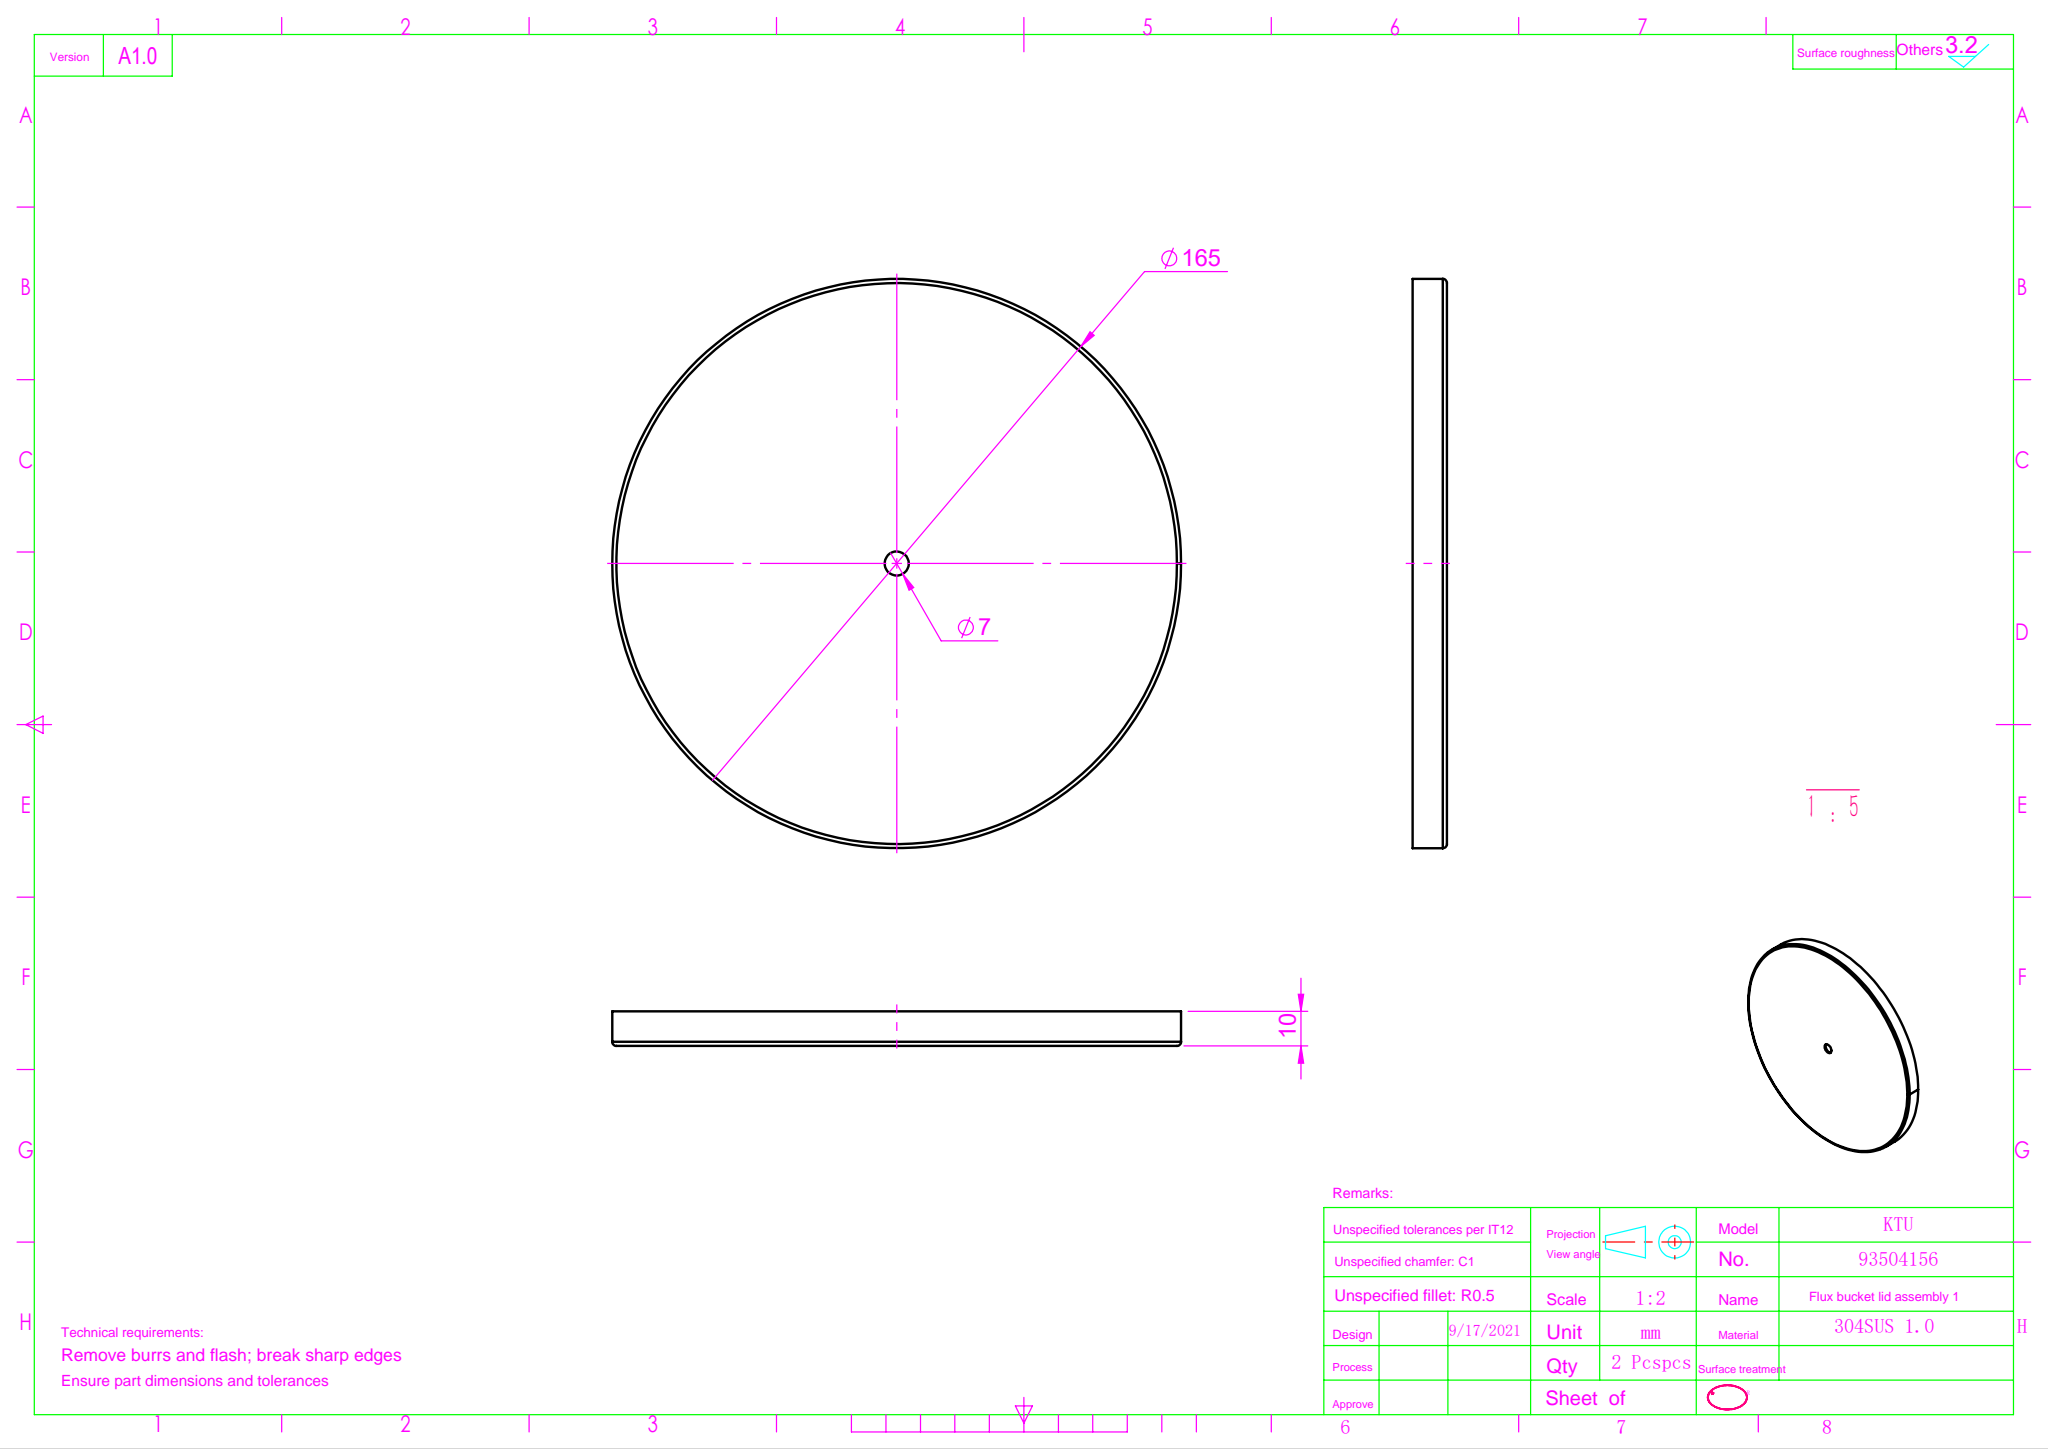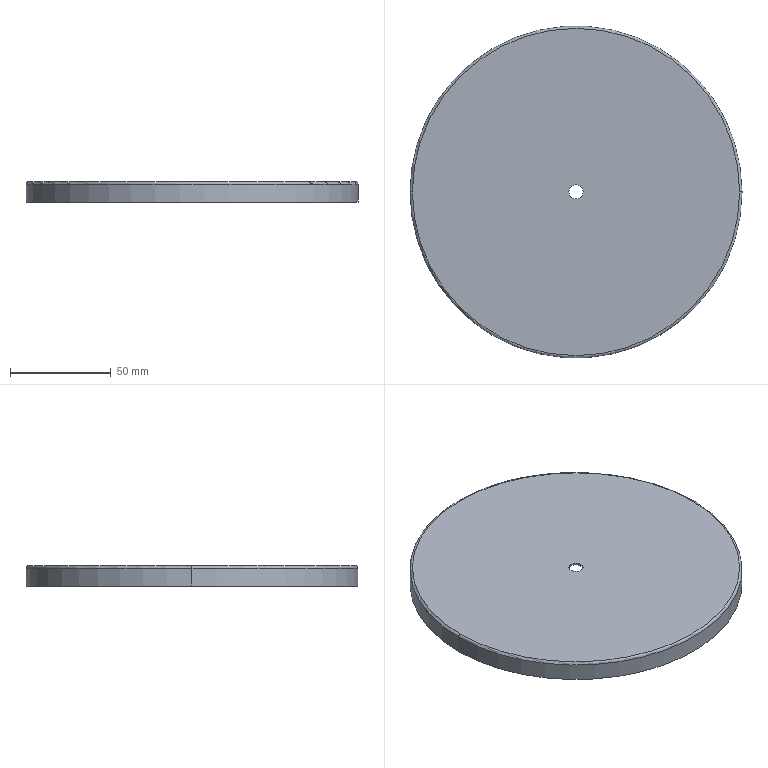Part | SolidWorks | features 3DProfileFeature 1, EdgeFlange 1, FlatPattern 1, ICE 1, SMBaseFlange 1, SheetMetal 1 | 1 solid | 13 faces | box 165 x 165 x 10 mm | volume 25826 mm3 | cylinder 6 | torus 4 | plane 3 | commonest cylinder face diameters 7 x2 163 x2 165 x2
STEP:
#1=CARTESIAN_POINT('',(-3.5,0.,-1.));
#2=VERTEX_POINT('',#1);
#3=CARTESIAN_POINT('',(3.5,0.,-1.));
#4=VERTEX_POINT('',#3);
#5=CARTESIAN_POINT('',(0.,0.,-1.));
#6=DIRECTION('',(0.,0.,1.));
#7=DIRECTION('',(1.,0.,0.));
#8=AXIS2_PLACEMENT_3D('',#5,#6,#7);
#9=CIRCLE('',#8,3.5);
#10=EDGE_CURVE('',#2,#4,#9,.T.);
#11=ORIENTED_EDGE('',*,*,#10,.F.);
#12=CARTESIAN_POINT('',(-3.5,0.,0.));
#13=VERTEX_POINT('',#12);
#14=CARTESIAN_POINT('',(-3.5,0.,-10.));
#15=DIRECTION('',(0.,0.,1.));
#16=VECTOR('',#15,1000.);
#17=LINE('',#14,#16);
#18=EDGE_CURVE('',#2,#13,#17,.T.);
#19=ORIENTED_EDGE('',*,*,#18,.T.);
#20=CARTESIAN_POINT('',(3.5,0.,0.));
#21=VERTEX_POINT('',#20);
#22=CARTESIAN_POINT('',(0.,0.,0.));
#23=DIRECTION('',(0.,0.,1.));
#24=DIRECTION('',(1.,0.,0.));
#25=AXIS2_PLACEMENT_3D('',#22,#23,#24);
#26=CIRCLE('',#25,3.5);
#27=EDGE_CURVE('',#13,#21,#26,.T.);
#28=ORIENTED_EDGE('',*,*,#27,.T.);
#29=CARTESIAN_POINT('',(3.5,0.,-10.));
#30=DIRECTION('',(0.,0.,1.));
#31=VECTOR('',#30,1000.);
#32=LINE('',#29,#31);
#33=EDGE_CURVE('',#4,#21,#32,.T.);
#34=ORIENTED_EDGE('',*,*,#33,.F.);
#35=EDGE_LOOP('',(#11,#19,#28,#34));
#36=FACE_OUTER_BOUND('',#35,.T.);
#37=CARTESIAN_POINT('',(0.,0.,-10.));
#38=DIRECTION('',(0.,0.,1.));
#39=DIRECTION('',(1.,0.,0.));
#40=AXIS2_PLACEMENT_3D('',#37,#38,#39);
#41=CYLINDRICAL_SURFACE('',#40,3.5);
#42=ADVANCED_FACE('',(#36),#41,.F.);
#43=CARTESIAN_POINT('',(-81.5,0.,-1.2));
#44=VERTEX_POINT('',#43);
#45=CARTESIAN_POINT('',(81.5,0.,-1.2));
#46=VERTEX_POINT('',#45);
#47=CARTESIAN_POINT('',(0.,0.,-1.2));
#48=DIRECTION('',(0.,0.,1.));
#49=DIRECTION('',(1.,0.,0.));
#50=AXIS2_PLACEMENT_3D('',#47,#48,#49);
#51=CIRCLE('',#50,81.5);
#52=EDGE_CURVE('',#44,#46,#51,.T.);
#53=ORIENTED_EDGE('',*,*,#52,.F.);
#54=CARTESIAN_POINT('',(-81.3,0.,-1.));
#55=VERTEX_POINT('',#54);
#56=CARTESIAN_POINT('',(-81.3,0.,-1.2));
#57=DIRECTION('',(0.,1.,0.));
#58=DIRECTION('',(-1.,0.,0.));
#59=AXIS2_PLACEMENT_3D('',#56,#57,#58);
#60=CIRCLE('',#59,0.2);
#61=EDGE_CURVE('',#44,#55,#60,.T.);
#62=ORIENTED_EDGE('',*,*,#61,.T.);
#63=CARTESIAN_POINT('',(81.3,0.,-1.));
#64=VERTEX_POINT('',#63);
#65=CARTESIAN_POINT('',(0.,0.,-1.));
#66=DIRECTION('',(0.,0.,1.));
#67=DIRECTION('',(1.,0.,0.));
#68=AXIS2_PLACEMENT_3D('',#65,#66,#67);
#69=CIRCLE('',#68,81.3);
#70=EDGE_CURVE('',#55,#64,#69,.T.);
#71=ORIENTED_EDGE('',*,*,#70,.T.);
#72=CARTESIAN_POINT('',(81.3,0.,-1.2));
#73=DIRECTION('',(0.,-1.,0.));
#74=DIRECTION('',(0.,0.,-1.));
#75=AXIS2_PLACEMENT_3D('',#72,#73,#74);
#76=CIRCLE('',#75,0.2);
#77=EDGE_CURVE('',#46,#64,#76,.T.);
#78=ORIENTED_EDGE('',*,*,#77,.F.);
#79=EDGE_LOOP('',(#53,#62,#71,#78));
#80=FACE_OUTER_BOUND('',#79,.T.);
#81=CARTESIAN_POINT('',(0.,0.,-1.2));
#82=DIRECTION('',(0.,0.,1.));
#83=DIRECTION('',(1.,0.,0.));
#84=AXIS2_PLACEMENT_3D('',#81,#82,#83);
#85=TOROIDAL_SURFACE('',#84,81.3,0.2);
#86=ADVANCED_FACE('',(#80),#85,.F.);
#87=CARTESIAN_POINT('',(-81.5,0.,-10.));
#88=VERTEX_POINT('',#87);
#89=CARTESIAN_POINT('',(81.5,0.,-10.));
#90=VERTEX_POINT('',#89);
#91=CARTESIAN_POINT('',(0.,0.,-10.));
#92=DIRECTION('',(0.,0.,1.));
#93=DIRECTION('',(1.,0.,0.));
#94=AXIS2_PLACEMENT_3D('',#91,#92,#93);
#95=CIRCLE('',#94,81.5);
#96=EDGE_CURVE('',#88,#90,#95,.T.);
#97=ORIENTED_EDGE('',*,*,#96,.F.);
#98=CARTESIAN_POINT('',(-81.5,0.,-1.));
#99=DIRECTION('',(0.,0.,1.));
#100=VECTOR('',#99,1000.);
#101=LINE('',#98,#100);
#102=EDGE_CURVE('',#88,#44,#101,.T.);
#103=ORIENTED_EDGE('',*,*,#102,.T.);
#104=ORIENTED_EDGE('',*,*,#52,.T.);
#105=CARTESIAN_POINT('',(81.5,0.,-1.));
#106=DIRECTION('',(0.,0.,1.));
#107=VECTOR('',#106,1000.);
#108=LINE('',#105,#107);
#109=EDGE_CURVE('',#90,#46,#108,.T.);
#110=ORIENTED_EDGE('',*,*,#109,.F.);
#111=EDGE_LOOP('',(#97,#103,#104,#110));
#112=FACE_OUTER_BOUND('',#111,.T.);
#113=CARTESIAN_POINT('',(0.,0.,-1.));
#114=DIRECTION('',(0.,0.,1.));
#115=DIRECTION('',(1.,0.,0.));
#116=AXIS2_PLACEMENT_3D('',#113,#114,#115);
#117=CYLINDRICAL_SURFACE('',#116,81.5);
#118=ADVANCED_FACE('',(#112),#117,.F.);
#119=CARTESIAN_POINT('',(82.5,0.,-1.2));
#120=VERTEX_POINT('',#119);
#121=CARTESIAN_POINT('',(-82.5,0.,-1.2));
#122=VERTEX_POINT('',#121);
#123=CARTESIAN_POINT('',(0.,0.,-1.2));
#124=DIRECTION('',(0.,0.,1.));
#125=DIRECTION('',(1.,0.,0.));
#126=AXIS2_PLACEMENT_3D('',#123,#124,#125);
#127=CIRCLE('',#126,82.5);
#128=EDGE_CURVE('',#120,#122,#127,.T.);
#129=ORIENTED_EDGE('',*,*,#128,.T.);
#130=CARTESIAN_POINT('',(-81.3,0.,0.));
#131=VERTEX_POINT('',#130);
#132=CARTESIAN_POINT('',(-81.3,0.,-1.2));
#133=DIRECTION('',(0.,1.,0.));
#134=DIRECTION('',(-1.,0.,0.));
#135=AXIS2_PLACEMENT_3D('',#132,#133,#134);
#136=CIRCLE('',#135,1.2);
#137=EDGE_CURVE('',#122,#131,#136,.T.);
#138=ORIENTED_EDGE('',*,*,#137,.T.);
#139=CARTESIAN_POINT('',(81.3,0.,0.));
#140=VERTEX_POINT('',#139);
#141=CARTESIAN_POINT('',(0.,0.,0.));
#142=DIRECTION('',(0.,0.,-1.));
#143=DIRECTION('',(1.,0.,0.));
#144=AXIS2_PLACEMENT_3D('',#141,#142,#143);
#145=CIRCLE('',#144,81.3);
#146=EDGE_CURVE('',#131,#140,#145,.T.);
#147=ORIENTED_EDGE('',*,*,#146,.T.);
#148=CARTESIAN_POINT('',(81.3,0.,-1.2));
#149=DIRECTION('',(0.,-1.,0.));
#150=DIRECTION('',(0.,0.,-1.));
#151=AXIS2_PLACEMENT_3D('',#148,#149,#150);
#152=CIRCLE('',#151,1.2);
#153=EDGE_CURVE('',#120,#140,#152,.T.);
#154=ORIENTED_EDGE('',*,*,#153,.F.);
#155=EDGE_LOOP('',(#129,#138,#147,#154));
#156=FACE_OUTER_BOUND('',#155,.T.);
#157=CARTESIAN_POINT('',(0.,0.,-1.2));
#158=DIRECTION('',(0.,0.,1.));
#159=DIRECTION('',(1.,0.,0.));
#160=AXIS2_PLACEMENT_3D('',#157,#158,#159);
#161=TOROIDAL_SURFACE('',#160,81.3,1.2);
#162=ADVANCED_FACE('',(#156),#161,.T.);
#163=CARTESIAN_POINT('',(82.5,0.,-10.));
#164=VERTEX_POINT('',#163);
#165=CARTESIAN_POINT('',(-82.5,0.,-10.));
#166=VERTEX_POINT('',#165);
#167=CARTESIAN_POINT('',(0.,0.,-10.));
#168=DIRECTION('',(0.,0.,1.));
#169=DIRECTION('',(1.,0.,0.));
#170=AXIS2_PLACEMENT_3D('',#167,#168,#169);
#171=CIRCLE('',#170,82.5);
#172=EDGE_CURVE('',#164,#166,#171,.T.);
#173=ORIENTED_EDGE('',*,*,#172,.T.);
#174=CARTESIAN_POINT('',(-82.5,0.,-1.));
#175=DIRECTION('',(0.,0.,1.));
#176=VECTOR('',#175,1000.);
#177=LINE('',#174,#176);
#178=EDGE_CURVE('',#166,#122,#177,.T.);
#179=ORIENTED_EDGE('',*,*,#178,.T.);
#180=ORIENTED_EDGE('',*,*,#128,.F.);
#181=CARTESIAN_POINT('',(82.5,0.,-1.));
#182=DIRECTION('',(0.,0.,1.));
#183=VECTOR('',#182,1000.);
#184=LINE('',#181,#183);
#185=EDGE_CURVE('',#164,#120,#184,.T.);
#186=ORIENTED_EDGE('',*,*,#185,.F.);
#187=EDGE_LOOP('',(#173,#179,#180,#186));
#188=FACE_OUTER_BOUND('',#187,.T.);
#189=CARTESIAN_POINT('',(0.,0.,-1.));
#190=DIRECTION('',(0.,0.,1.));
#191=DIRECTION('',(1.,0.,0.));
#192=AXIS2_PLACEMENT_3D('',#189,#190,#191);
#193=CYLINDRICAL_SURFACE('',#192,82.5);
#194=ADVANCED_FACE('',(#188),#193,.T.);
#195=CARTESIAN_POINT('',(0.,0.,-1.));
#196=DIRECTION('',(0.,0.,1.));
#197=DIRECTION('',(1.,0.,0.));
#198=AXIS2_PLACEMENT_3D('',#195,#196,#197);
#199=CIRCLE('',#198,3.5);
#200=EDGE_CURVE('',#4,#2,#199,.T.);
#201=ORIENTED_EDGE('',*,*,#200,.T.);
#202=ORIENTED_EDGE('',*,*,#10,.T.);
#203=EDGE_LOOP('',(#201,#202));
#204=FACE_BOUND('',#203,.T.);
#205=CARTESIAN_POINT('',(0.,0.,-1.));
#206=DIRECTION('',(0.,0.,1.));
#207=DIRECTION('',(1.,0.,0.));
#208=AXIS2_PLACEMENT_3D('',#205,#206,#207);
#209=CIRCLE('',#208,81.3);
#210=EDGE_CURVE('',#64,#55,#209,.T.);
#211=ORIENTED_EDGE('',*,*,#210,.F.);
#212=ORIENTED_EDGE('',*,*,#70,.F.);
#213=EDGE_LOOP('',(#211,#212));
#214=FACE_OUTER_BOUND('',#213,.T.);
#215=CARTESIAN_POINT('',(0.,0.,-1.));
#216=DIRECTION('',(0.,0.,1.));
#217=DIRECTION('',(1.,0.,0.));
#218=AXIS2_PLACEMENT_3D('',#215,#216,#217);
#219=PLANE('',#218);
#220=ADVANCED_FACE('',(#204,#214),#219,.F.);
#221=ORIENTED_EDGE('',*,*,#172,.F.);
#222=CARTESIAN_POINT('',(0.,0.,-10.));
#223=DIRECTION('',(0.,0.,1.));
#224=DIRECTION('',(1.,0.,0.));
#225=AXIS2_PLACEMENT_3D('',#222,#223,#224);
#226=CIRCLE('',#225,82.5);
#227=EDGE_CURVE('',#166,#164,#226,.T.);
#228=ORIENTED_EDGE('',*,*,#227,.F.);
#229=EDGE_LOOP('',(#221,#228));
#230=FACE_OUTER_BOUND('',#229,.T.);
#231=CARTESIAN_POINT('',(0.,0.,-10.));
#232=DIRECTION('',(0.,0.,1.));
#233=DIRECTION('',(1.,0.,0.));
#234=AXIS2_PLACEMENT_3D('',#231,#232,#233);
#235=CIRCLE('',#234,81.5);
#236=EDGE_CURVE('',#90,#88,#235,.T.);
#237=ORIENTED_EDGE('',*,*,#236,.T.);
#238=ORIENTED_EDGE('',*,*,#96,.T.);
#239=EDGE_LOOP('',(#237,#238));
#240=FACE_BOUND('',#239,.T.);
#241=CARTESIAN_POINT('',(0.,0.,-10.));
#242=DIRECTION('',(0.,0.,-1.));
#243=DIRECTION('',(-1.,0.,0.));
#244=AXIS2_PLACEMENT_3D('',#241,#242,#243);
#245=PLANE('',#244);
#246=ADVANCED_FACE('',(#230,#240),#245,.T.);
#247=ORIENTED_EDGE('',*,*,#178,.F.);
#248=ORIENTED_EDGE('',*,*,#227,.T.);
#249=ORIENTED_EDGE('',*,*,#185,.T.);
#250=CARTESIAN_POINT('',(0.,0.,-1.2));
#251=DIRECTION('',(0.,0.,1.));
#252=DIRECTION('',(1.,0.,0.));
#253=AXIS2_PLACEMENT_3D('',#250,#251,#252);
#254=CIRCLE('',#253,82.5);
#255=EDGE_CURVE('',#122,#120,#254,.T.);
#256=ORIENTED_EDGE('',*,*,#255,.F.);
#257=EDGE_LOOP('',(#247,#248,#249,#256));
#258=FACE_OUTER_BOUND('',#257,.T.);
#259=CARTESIAN_POINT('',(0.,0.,-1.));
#260=DIRECTION('',(0.,0.,1.));
#261=DIRECTION('',(1.,0.,0.));
#262=AXIS2_PLACEMENT_3D('',#259,#260,#261);
#263=CYLINDRICAL_SURFACE('',#262,82.5);
#264=ADVANCED_FACE('',(#258),#263,.T.);
#265=ORIENTED_EDGE('',*,*,#137,.F.);
#266=ORIENTED_EDGE('',*,*,#255,.T.);
#267=ORIENTED_EDGE('',*,*,#153,.T.);
#268=CARTESIAN_POINT('',(0.,0.,0.));
#269=DIRECTION('',(0.,0.,-1.));
#270=DIRECTION('',(1.,0.,0.));
#271=AXIS2_PLACEMENT_3D('',#268,#269,#270);
#272=CIRCLE('',#271,81.3);
#273=EDGE_CURVE('',#140,#131,#272,.T.);
#274=ORIENTED_EDGE('',*,*,#273,.T.);
#275=EDGE_LOOP('',(#265,#266,#267,#274));
#276=FACE_OUTER_BOUND('',#275,.T.);
#277=CARTESIAN_POINT('',(0.,0.,-1.2));
#278=DIRECTION('',(0.,0.,1.));
#279=DIRECTION('',(1.,0.,0.));
#280=AXIS2_PLACEMENT_3D('',#277,#278,#279);
#281=TOROIDAL_SURFACE('',#280,81.3,1.2);
#282=ADVANCED_FACE('',(#276),#281,.T.);
#283=ORIENTED_EDGE('',*,*,#102,.F.);
#284=ORIENTED_EDGE('',*,*,#236,.F.);
#285=ORIENTED_EDGE('',*,*,#109,.T.);
#286=CARTESIAN_POINT('',(0.,0.,-1.2));
#287=DIRECTION('',(0.,0.,1.));
#288=DIRECTION('',(1.,0.,0.));
#289=AXIS2_PLACEMENT_3D('',#286,#287,#288);
#290=CIRCLE('',#289,81.5);
#291=EDGE_CURVE('',#46,#44,#290,.T.);
#292=ORIENTED_EDGE('',*,*,#291,.T.);
#293=EDGE_LOOP('',(#283,#284,#285,#292));
#294=FACE_OUTER_BOUND('',#293,.T.);
#295=CARTESIAN_POINT('',(0.,0.,-1.));
#296=DIRECTION('',(0.,0.,1.));
#297=DIRECTION('',(1.,0.,0.));
#298=AXIS2_PLACEMENT_3D('',#295,#296,#297);
#299=CYLINDRICAL_SURFACE('',#298,81.5);
#300=ADVANCED_FACE('',(#294),#299,.F.);
#301=ORIENTED_EDGE('',*,*,#61,.F.);
#302=ORIENTED_EDGE('',*,*,#291,.F.);
#303=ORIENTED_EDGE('',*,*,#77,.T.);
#304=ORIENTED_EDGE('',*,*,#210,.T.);
#305=EDGE_LOOP('',(#301,#302,#303,#304));
#306=FACE_OUTER_BOUND('',#305,.T.);
#307=CARTESIAN_POINT('',(0.,0.,-1.2));
#308=DIRECTION('',(0.,0.,1.));
#309=DIRECTION('',(1.,0.,0.));
#310=AXIS2_PLACEMENT_3D('',#307,#308,#309);
#311=TOROIDAL_SURFACE('',#310,81.3,0.2);
#312=ADVANCED_FACE('',(#306),#311,.F.);
#313=CARTESIAN_POINT('',(0.,0.,0.));
#314=DIRECTION('',(0.,0.,1.));
#315=DIRECTION('',(1.,0.,0.));
#316=AXIS2_PLACEMENT_3D('',#313,#314,#315);
#317=CIRCLE('',#316,3.5);
#318=EDGE_CURVE('',#21,#13,#317,.T.);
#319=ORIENTED_EDGE('',*,*,#318,.F.);
#320=ORIENTED_EDGE('',*,*,#27,.F.);
#321=EDGE_LOOP('',(#319,#320));
#322=FACE_BOUND('',#321,.T.);
#323=ORIENTED_EDGE('',*,*,#273,.F.);
#324=ORIENTED_EDGE('',*,*,#146,.F.);
#325=EDGE_LOOP('',(#323,#324));
#326=FACE_OUTER_BOUND('',#325,.T.);
#327=CARTESIAN_POINT('',(0.,0.,0.));
#328=DIRECTION('',(0.,0.,1.));
#329=DIRECTION('',(1.,0.,0.));
#330=AXIS2_PLACEMENT_3D('',#327,#328,#329);
#331=PLANE('',#330);
#332=ADVANCED_FACE('',(#322,#326),#331,.T.);
#333=ORIENTED_EDGE('',*,*,#18,.F.);
#334=ORIENTED_EDGE('',*,*,#200,.F.);
#335=ORIENTED_EDGE('',*,*,#33,.T.);
#336=ORIENTED_EDGE('',*,*,#318,.T.);
#337=EDGE_LOOP('',(#333,#334,#335,#336));
#338=FACE_OUTER_BOUND('',#337,.T.);
#339=CARTESIAN_POINT('',(0.,0.,-10.));
#340=DIRECTION('',(0.,0.,1.));
#341=DIRECTION('',(1.,0.,0.));
#342=AXIS2_PLACEMENT_3D('',#339,#340,#341);
#343=CYLINDRICAL_SURFACE('',#342,3.5);
#344=ADVANCED_FACE('',(#338),#343,.F.);
#345=CLOSED_SHELL('',(#42,#86,#118,#162,#194,#220,#246,#264,#282,#300,#312,#332,#344));
#346=MANIFOLD_SOLID_BREP('',#345);
#347=CARTESIAN_POINT('',(0.,0.,0.));
#348=DIRECTION('',(0.,0.,1.));
#349=DIRECTION('',(1.,0.,0.));
#350=AXIS2_PLACEMENT_3D('',#347,#348,#349);
#351=(LENGTH_UNIT()NAMED_UNIT(*)SI_UNIT(.MILLI.,.METRE.));
#352=UNCERTAINTY_MEASURE_WITH_UNIT(LENGTH_MEASURE(0.00001),#351,'','');
#353=(NAMED_UNIT(*)PLANE_ANGLE_UNIT()SI_UNIT($,.RADIAN.));
#354=(NAMED_UNIT(*)SI_UNIT($,.STERADIAN.)SOLID_ANGLE_UNIT());
#355=(GEOMETRIC_REPRESENTATION_CONTEXT(3)GLOBAL_UNCERTAINTY_ASSIGNED_CONTEXT((#352))GLOBAL_UNIT_ASSIGNED_CONTEXT((#351,#353,#354))REPRESENTATION_CONTEXT('',''));
#356=ADVANCED_BREP_SHAPE_REPRESENTATION('',(#346,#350),#355);